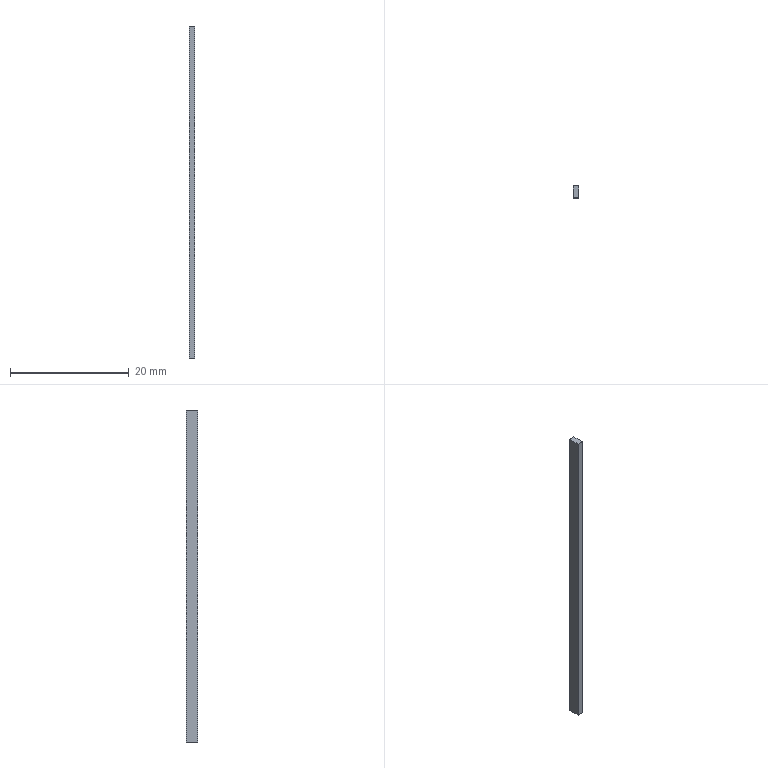Part | NX | features BREP 2 | 2 solids | 12 faces | box 0.9799 x 2 x 56 mm | volume 219.497 mm3 | plane 12
STEP:
#1=CARTESIAN_POINT('',(0.5149,1.025,-4.));
#2=VERTEX_POINT('',#1);
#3=CARTESIAN_POINT('',(0.5149,1.025,52.));
#4=VERTEX_POINT('',#3);
#5=CARTESIAN_POINT('',(0.5149,1.025,0.));
#6=DIRECTION('',(0.,0.,1.));
#7=VECTOR('',#6,1000.);
#8=LINE('',#5,#7);
#9=EDGE_CURVE('',#2,#4,#8,.T.);
#10=ORIENTED_EDGE('',*,*,#9,.T.);
#11=CARTESIAN_POINT('',(0.5149,-0.975,52.));
#12=VERTEX_POINT('',#11);
#13=CARTESIAN_POINT('',(0.5149,-12.681,52.));
#14=DIRECTION('',(0.,1.,0.));
#15=VECTOR('',#14,1000.);
#16=LINE('',#13,#15);
#17=EDGE_CURVE('',#12,#4,#16,.T.);
#18=ORIENTED_EDGE('',*,*,#17,.F.);
#19=CARTESIAN_POINT('',(0.5149,-0.975,-4.));
#20=VERTEX_POINT('',#19);
#21=CARTESIAN_POINT('',(0.5149,-0.975,0.));
#22=DIRECTION('',(0.,0.,1.));
#23=VECTOR('',#22,1000.);
#24=LINE('',#21,#23);
#25=EDGE_CURVE('',#20,#12,#24,.T.);
#26=ORIENTED_EDGE('',*,*,#25,.F.);
#27=CARTESIAN_POINT('',(0.5149,-12.681,-4.));
#28=DIRECTION('',(0.,1.,0.));
#29=VECTOR('',#28,1000.);
#30=LINE('',#27,#29);
#31=EDGE_CURVE('',#20,#2,#30,.T.);
#32=ORIENTED_EDGE('',*,*,#31,.T.);
#33=EDGE_LOOP('',(#10,#18,#26,#32));
#34=FACE_BOUND('',#33,.T.);
#35=CARTESIAN_POINT('',(0.5149,1.718,0.));
#36=DIRECTION('',(-1.,0.,0.));
#37=DIRECTION('',(0.,1.,0.));
#38=AXIS2_PLACEMENT_3D('',#35,#36,#37);
#39=PLANE('',#38);
#40=ADVANCED_FACE('',(#34),#39,.F.);
#41=ORIENTED_EDGE('',*,*,#25,.T.);
#42=CARTESIAN_POINT('',(-0.465,-0.975,52.));
#43=VERTEX_POINT('',#42);
#44=CARTESIAN_POINT('',(-7.015,-0.975,52.));
#45=DIRECTION('',(1.,0.,0.));
#46=VECTOR('',#45,1000.);
#47=LINE('',#44,#46);
#48=EDGE_CURVE('',#43,#12,#47,.T.);
#49=ORIENTED_EDGE('',*,*,#48,.F.);
#50=CARTESIAN_POINT('',(-0.465,-0.975,-4.));
#51=VERTEX_POINT('',#50);
#52=CARTESIAN_POINT('',(-0.465,-0.975,0.));
#53=DIRECTION('',(0.,0.,1.));
#54=VECTOR('',#53,1000.);
#55=LINE('',#52,#54);
#56=EDGE_CURVE('',#51,#43,#55,.T.);
#57=ORIENTED_EDGE('',*,*,#56,.F.);
#58=CARTESIAN_POINT('',(-7.015,-0.975,-4.));
#59=DIRECTION('',(1.,0.,0.));
#60=VECTOR('',#59,1000.);
#61=LINE('',#58,#60);
#62=EDGE_CURVE('',#51,#20,#61,.T.);
#63=ORIENTED_EDGE('',*,*,#62,.T.);
#64=EDGE_LOOP('',(#41,#49,#57,#63));
#65=FACE_BOUND('',#64,.T.);
#66=CARTESIAN_POINT('',(-7.015,-0.975,0.));
#67=DIRECTION('',(0.,-1.,0.));
#68=DIRECTION('',(-1.,0.,0.));
#69=AXIS2_PLACEMENT_3D('',#66,#67,#68);
#70=PLANE('',#69);
#71=ADVANCED_FACE('',(#65),#70,.T.);
#72=ORIENTED_EDGE('',*,*,#56,.T.);
#73=CARTESIAN_POINT('',(-0.465,1.025,52.));
#74=VERTEX_POINT('',#73);
#75=CARTESIAN_POINT('',(-0.465,-12.681,52.));
#76=DIRECTION('',(0.,-1.,0.));
#77=VECTOR('',#76,1000.);
#78=LINE('',#75,#77);
#79=EDGE_CURVE('',#74,#43,#78,.T.);
#80=ORIENTED_EDGE('',*,*,#79,.F.);
#81=CARTESIAN_POINT('',(-0.465,1.025,-4.));
#82=VERTEX_POINT('',#81);
#83=CARTESIAN_POINT('',(-0.465,1.025,0.));
#84=DIRECTION('',(0.,0.,1.));
#85=VECTOR('',#84,1000.);
#86=LINE('',#83,#85);
#87=EDGE_CURVE('',#82,#74,#86,.T.);
#88=ORIENTED_EDGE('',*,*,#87,.F.);
#89=CARTESIAN_POINT('',(-0.465,-12.681,-4.));
#90=DIRECTION('',(0.,-1.,0.));
#91=VECTOR('',#90,1000.);
#92=LINE('',#89,#91);
#93=EDGE_CURVE('',#82,#51,#92,.T.);
#94=ORIENTED_EDGE('',*,*,#93,.T.);
#95=EDGE_LOOP('',(#72,#80,#88,#94));
#96=FACE_BOUND('',#95,.T.);
#97=CARTESIAN_POINT('',(-0.465,-0.975,0.));
#98=DIRECTION('',(1.,0.,0.));
#99=DIRECTION('',(0.,-1.,0.));
#100=AXIS2_PLACEMENT_3D('',#97,#98,#99);
#101=PLANE('',#100);
#102=ADVANCED_FACE('',(#96),#101,.F.);
#103=CARTESIAN_POINT('',(-7.015,1.025,-4.));
#104=DIRECTION('',(-1.,0.,0.));
#105=VECTOR('',#104,1000.);
#106=LINE('',#103,#105);
#107=EDGE_CURVE('',#2,#82,#106,.T.);
#108=ORIENTED_EDGE('',*,*,#107,.T.);
#109=ORIENTED_EDGE('',*,*,#87,.T.);
#110=CARTESIAN_POINT('',(-7.015,1.025,52.));
#111=DIRECTION('',(-1.,0.,0.));
#112=VECTOR('',#111,1000.);
#113=LINE('',#110,#112);
#114=EDGE_CURVE('',#4,#74,#113,.T.);
#115=ORIENTED_EDGE('',*,*,#114,.F.);
#116=ORIENTED_EDGE('',*,*,#9,.F.);
#117=EDGE_LOOP('',(#108,#109,#115,#116));
#118=FACE_BOUND('',#117,.T.);
#119=CARTESIAN_POINT('',(-7.015,1.025,0.));
#120=DIRECTION('',(0.,-1.,0.));
#121=DIRECTION('',(-1.,0.,0.));
#122=AXIS2_PLACEMENT_3D('',#119,#120,#121);
#123=PLANE('',#122);
#124=ADVANCED_FACE('',(#118),#123,.F.);
#125=ORIENTED_EDGE('',*,*,#79,.T.);
#126=ORIENTED_EDGE('',*,*,#48,.T.);
#127=ORIENTED_EDGE('',*,*,#17,.T.);
#128=ORIENTED_EDGE('',*,*,#114,.T.);
#129=EDGE_LOOP('',(#125,#126,#127,#128));
#130=FACE_BOUND('',#129,.T.);
#131=CARTESIAN_POINT('',(-7.015,-12.681,52.));
#132=DIRECTION('',(0.,0.,1.));
#133=DIRECTION('',(-1.,0.,0.));
#134=AXIS2_PLACEMENT_3D('',#131,#132,#133);
#135=PLANE('',#134);
#136=ADVANCED_FACE('',(#130),#135,.T.);
#137=ORIENTED_EDGE('',*,*,#93,.F.);
#138=ORIENTED_EDGE('',*,*,#107,.F.);
#139=ORIENTED_EDGE('',*,*,#31,.F.);
#140=ORIENTED_EDGE('',*,*,#62,.F.);
#141=EDGE_LOOP('',(#137,#138,#139,#140));
#142=FACE_BOUND('',#141,.T.);
#143=CARTESIAN_POINT('',(-7.015,-12.681,-4.));
#144=DIRECTION('',(0.,0.,1.));
#145=DIRECTION('',(-1.,0.,0.));
#146=AXIS2_PLACEMENT_3D('',#143,#144,#145);
#147=PLANE('',#146);
#148=ADVANCED_FACE('',(#142),#147,.F.);
#149=CLOSED_SHELL('',(#40,#71,#102,#124,#136,#148));
#150=MANIFOLD_SOLID_BREP('',#149);
#151=CARTESIAN_POINT('',(0.5149,1.025,-4.));
#152=VERTEX_POINT('',#151);
#153=CARTESIAN_POINT('',(0.5149,1.025,52.));
#154=VERTEX_POINT('',#153);
#155=CARTESIAN_POINT('',(0.5149,1.025,0.));
#156=DIRECTION('',(0.,0.,1.));
#157=VECTOR('',#156,1000.);
#158=LINE('',#155,#157);
#159=EDGE_CURVE('',#152,#154,#158,.T.);
#160=ORIENTED_EDGE('',*,*,#159,.T.);
#161=CARTESIAN_POINT('',(0.5149,-0.975,52.));
#162=VERTEX_POINT('',#161);
#163=CARTESIAN_POINT('',(0.5149,-12.681,52.));
#164=DIRECTION('',(0.,1.,0.));
#165=VECTOR('',#164,1000.);
#166=LINE('',#163,#165);
#167=EDGE_CURVE('',#162,#154,#166,.T.);
#168=ORIENTED_EDGE('',*,*,#167,.F.);
#169=CARTESIAN_POINT('',(0.5149,-0.975,-4.));
#170=VERTEX_POINT('',#169);
#171=CARTESIAN_POINT('',(0.5149,-0.975,0.));
#172=DIRECTION('',(0.,0.,1.));
#173=VECTOR('',#172,1000.);
#174=LINE('',#171,#173);
#175=EDGE_CURVE('',#170,#162,#174,.T.);
#176=ORIENTED_EDGE('',*,*,#175,.F.);
#177=CARTESIAN_POINT('',(0.5149,-12.681,-4.));
#178=DIRECTION('',(0.,1.,0.));
#179=VECTOR('',#178,1000.);
#180=LINE('',#177,#179);
#181=EDGE_CURVE('',#170,#152,#180,.T.);
#182=ORIENTED_EDGE('',*,*,#181,.T.);
#183=EDGE_LOOP('',(#160,#168,#176,#182));
#184=FACE_BOUND('',#183,.T.);
#185=CARTESIAN_POINT('',(0.5149,1.718,0.));
#186=DIRECTION('',(-1.,0.,0.));
#187=DIRECTION('',(0.,1.,0.));
#188=AXIS2_PLACEMENT_3D('',#185,#186,#187);
#189=PLANE('',#188);
#190=ADVANCED_FACE('',(#184),#189,.F.);
#191=ORIENTED_EDGE('',*,*,#175,.T.);
#192=CARTESIAN_POINT('',(-0.465,-0.975,52.));
#193=VERTEX_POINT('',#192);
#194=CARTESIAN_POINT('',(-7.015,-0.975,52.));
#195=DIRECTION('',(1.,0.,0.));
#196=VECTOR('',#195,1000.);
#197=LINE('',#194,#196);
#198=EDGE_CURVE('',#193,#162,#197,.T.);
#199=ORIENTED_EDGE('',*,*,#198,.F.);
#200=CARTESIAN_POINT('',(-0.465,-0.975,-4.));
#201=VERTEX_POINT('',#200);
#202=CARTESIAN_POINT('',(-0.465,-0.975,0.));
#203=DIRECTION('',(0.,0.,1.));
#204=VECTOR('',#203,1000.);
#205=LINE('',#202,#204);
#206=EDGE_CURVE('',#201,#193,#205,.T.);
#207=ORIENTED_EDGE('',*,*,#206,.F.);
#208=CARTESIAN_POINT('',(-7.015,-0.975,-4.));
#209=DIRECTION('',(1.,0.,0.));
#210=VECTOR('',#209,1000.);
#211=LINE('',#208,#210);
#212=EDGE_CURVE('',#201,#170,#211,.T.);
#213=ORIENTED_EDGE('',*,*,#212,.T.);
#214=EDGE_LOOP('',(#191,#199,#207,#213));
#215=FACE_BOUND('',#214,.T.);
#216=CARTESIAN_POINT('',(-7.015,-0.975,0.));
#217=DIRECTION('',(0.,-1.,0.));
#218=DIRECTION('',(-1.,0.,0.));
#219=AXIS2_PLACEMENT_3D('',#216,#217,#218);
#220=PLANE('',#219);
#221=ADVANCED_FACE('',(#215),#220,.T.);
#222=ORIENTED_EDGE('',*,*,#206,.T.);
#223=CARTESIAN_POINT('',(-0.465,1.025,52.));
#224=VERTEX_POINT('',#223);
#225=CARTESIAN_POINT('',(-0.465,-12.681,52.));
#226=DIRECTION('',(0.,-1.,0.));
#227=VECTOR('',#226,1000.);
#228=LINE('',#225,#227);
#229=EDGE_CURVE('',#224,#193,#228,.T.);
#230=ORIENTED_EDGE('',*,*,#229,.F.);
#231=CARTESIAN_POINT('',(-0.465,1.025,-4.));
#232=VERTEX_POINT('',#231);
#233=CARTESIAN_POINT('',(-0.465,1.025,0.));
#234=DIRECTION('',(0.,0.,1.));
#235=VECTOR('',#234,1000.);
#236=LINE('',#233,#235);
#237=EDGE_CURVE('',#232,#224,#236,.T.);
#238=ORIENTED_EDGE('',*,*,#237,.F.);
#239=CARTESIAN_POINT('',(-0.465,-12.681,-4.));
#240=DIRECTION('',(0.,-1.,0.));
#241=VECTOR('',#240,1000.);
#242=LINE('',#239,#241);
#243=EDGE_CURVE('',#232,#201,#242,.T.);
#244=ORIENTED_EDGE('',*,*,#243,.T.);
#245=EDGE_LOOP('',(#222,#230,#238,#244));
#246=FACE_BOUND('',#245,.T.);
#247=CARTESIAN_POINT('',(-0.465,-0.975,0.));
#248=DIRECTION('',(1.,0.,0.));
#249=DIRECTION('',(0.,-1.,0.));
#250=AXIS2_PLACEMENT_3D('',#247,#248,#249);
#251=PLANE('',#250);
#252=ADVANCED_FACE('',(#246),#251,.F.);
#253=CARTESIAN_POINT('',(-7.015,1.025,-4.));
#254=DIRECTION('',(-1.,0.,0.));
#255=VECTOR('',#254,1000.);
#256=LINE('',#253,#255);
#257=EDGE_CURVE('',#152,#232,#256,.T.);
#258=ORIENTED_EDGE('',*,*,#257,.T.);
#259=ORIENTED_EDGE('',*,*,#237,.T.);
#260=CARTESIAN_POINT('',(-7.015,1.025,52.));
#261=DIRECTION('',(-1.,0.,0.));
#262=VECTOR('',#261,1000.);
#263=LINE('',#260,#262);
#264=EDGE_CURVE('',#154,#224,#263,.T.);
#265=ORIENTED_EDGE('',*,*,#264,.F.);
#266=ORIENTED_EDGE('',*,*,#159,.F.);
#267=EDGE_LOOP('',(#258,#259,#265,#266));
#268=FACE_BOUND('',#267,.T.);
#269=CARTESIAN_POINT('',(-7.015,1.025,0.));
#270=DIRECTION('',(0.,-1.,0.));
#271=DIRECTION('',(-1.,0.,0.));
#272=AXIS2_PLACEMENT_3D('',#269,#270,#271);
#273=PLANE('',#272);
#274=ADVANCED_FACE('',(#268),#273,.F.);
#275=ORIENTED_EDGE('',*,*,#229,.T.);
#276=ORIENTED_EDGE('',*,*,#198,.T.);
#277=ORIENTED_EDGE('',*,*,#167,.T.);
#278=ORIENTED_EDGE('',*,*,#264,.T.);
#279=EDGE_LOOP('',(#275,#276,#277,#278));
#280=FACE_BOUND('',#279,.T.);
#281=CARTESIAN_POINT('',(-7.015,-12.681,52.));
#282=DIRECTION('',(0.,0.,1.));
#283=DIRECTION('',(-1.,0.,0.));
#284=AXIS2_PLACEMENT_3D('',#281,#282,#283);
#285=PLANE('',#284);
#286=ADVANCED_FACE('',(#280),#285,.T.);
#287=ORIENTED_EDGE('',*,*,#243,.F.);
#288=ORIENTED_EDGE('',*,*,#257,.F.);
#289=ORIENTED_EDGE('',*,*,#181,.F.);
#290=ORIENTED_EDGE('',*,*,#212,.F.);
#291=EDGE_LOOP('',(#287,#288,#289,#290));
#292=FACE_BOUND('',#291,.T.);
#293=CARTESIAN_POINT('',(-7.015,-12.681,-4.));
#294=DIRECTION('',(0.,0.,1.));
#295=DIRECTION('',(-1.,0.,0.));
#296=AXIS2_PLACEMENT_3D('',#293,#294,#295);
#297=PLANE('',#296);
#298=ADVANCED_FACE('',(#292),#297,.F.);
#299=CLOSED_SHELL('',(#190,#221,#252,#274,#286,#298));
#300=MANIFOLD_SOLID_BREP('',#299);
#301=(LENGTH_UNIT()NAMED_UNIT(*)SI_UNIT(.MILLI.,.METRE.));
#302=UNCERTAINTY_MEASURE_WITH_UNIT(LENGTH_MEASURE(0.00001),#301,'','');
#303=(NAMED_UNIT(*)PLANE_ANGLE_UNIT()SI_UNIT($,.RADIAN.));
#304=(NAMED_UNIT(*)SI_UNIT($,.STERADIAN.)SOLID_ANGLE_UNIT());
#305=(GEOMETRIC_REPRESENTATION_CONTEXT(3)GLOBAL_UNCERTAINTY_ASSIGNED_CONTEXT((#302))GLOBAL_UNIT_ASSIGNED_CONTEXT((#301,#303,#304))REPRESENTATION_CONTEXT('',''));
#306=ADVANCED_BREP_SHAPE_REPRESENTATION('',(#150,#300),#305);